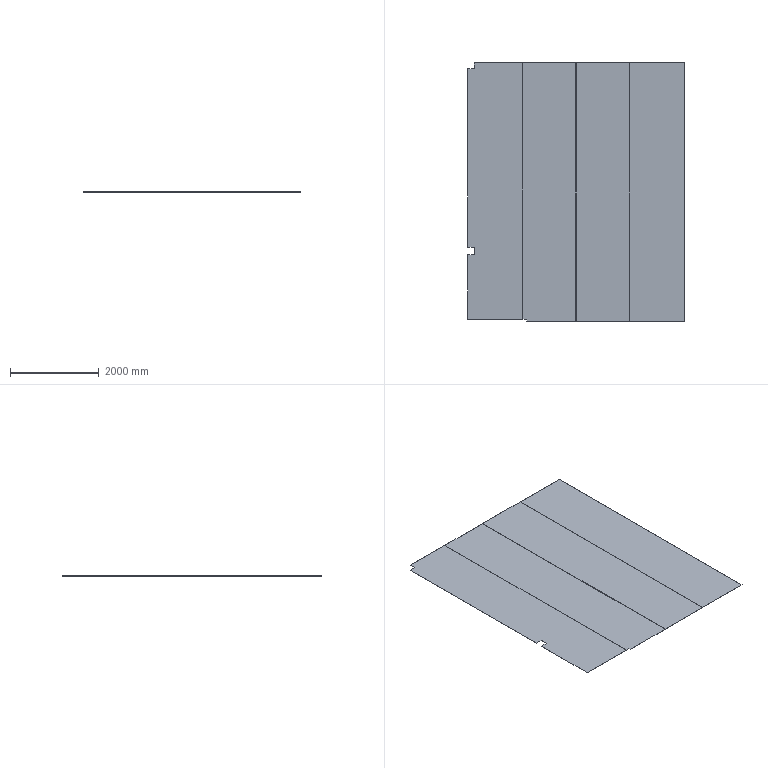Part | STEP file | 电柜花纹Plate | 4 solids | 32 faces | box 4900 x 5840 x 3 mm | volume 85436520 mm3 | plane 32